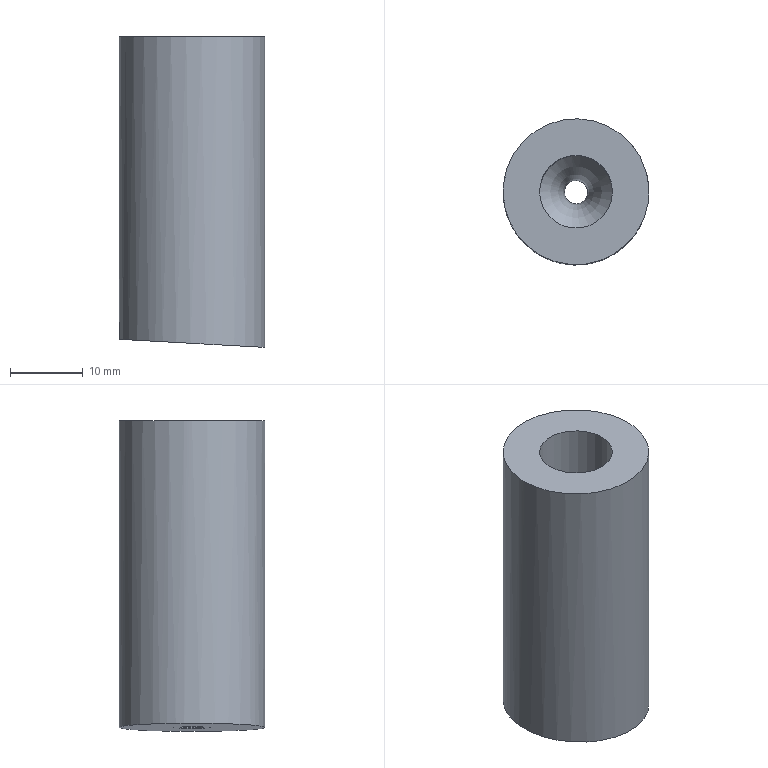Part | NX | features solid 2 | 1 solid | 7 faces | box 20 x 20 x 42.607 mm | volume 10571 mm3 | cylinder 3 | spline 2 | plane 1 | torus 1 | commonest cylinder face diameters 3.2 x1 10 x1 20 x1
STEP:
#1=CARTESIAN_POINT('',(262.245,42.7,-39.614));
#2=VERTEX_POINT('',#1);
#3=CARTESIAN_POINT('',(260.645,42.7,-39.614));
#4=DIRECTION('',(0.,0.,1.));
#5=DIRECTION('',(1.,0.,0.));
#6=AXIS2_PLACEMENT_3D('',#3,#4,#5);
#7=CIRCLE('',#6,1.6);
#8=EDGE_CURVE('',#2,#2,#7,.F.);
#9=ORIENTED_EDGE('',*,*,#8,.F.);
#10=EDGE_LOOP('',(#9));
#11=FACE_BOUND('',#10,.T.);
#12=CARTESIAN_POINT('',(260.645,44.3,-43.051));
#13=VERTEX_POINT('',#12);
#14=CARTESIAN_POINT('',(261.9,43.953,-43.121));
#15=CARTESIAN_POINT('',(260.645,44.473,-43.051));
#16=CARTESIAN_POINT('',(259.392,43.954,-42.982));
#17=CARTESIAN_POINT('',(258.872,42.701,-42.953));
#18=CARTESIAN_POINT('',(259.391,41.446,-42.982));
#19=CARTESIAN_POINT('',(260.645,40.927,-43.051));
#20=CARTESIAN_POINT('',(261.897,41.444,-43.121));
#21=CARTESIAN_POINT('',(262.419,42.698,-43.15));
#22=CARTESIAN_POINT('',(261.9,43.953,-43.121));
#23=CARTESIAN_POINT('',(260.645,44.473,-43.051));
#24=CARTESIAN_POINT('',(259.392,43.954,-42.982));
#25=B_SPLINE_CURVE_WITH_KNOTS('',3,(#14,#15,#16,#17,#18,#19,#20,#21,#22,#23,#24),.UNSPECIFIED.,.T.,.F.,(1,1,1,1,1,1,1,1,1,1,1,1,1,1,1),(-0.003754,-0.002503,-0.001251,0.,0.001251,0.002503,0.003754,0.005006,0.006257,0.007508,0.00876,0.01001,0.01126,0.01251,0.01377),.UNSPECIFIED.);
#26=EDGE_CURVE('',#13,#13,#25,.T.);
#27=ORIENTED_EDGE('',*,*,#26,.F.);
#28=EDGE_LOOP('',(#27));
#29=FACE_BOUND('',#28,.T.);
#30=CARTESIAN_POINT('',(260.645,42.7,-61.));
#31=DIRECTION('',(0.,0.,1.));
#32=DIRECTION('',(0.,1.,0.));
#33=AXIS2_PLACEMENT_3D('',#30,#31,#32);
#34=CYLINDRICAL_SURFACE('',#33,1.6);
#35=ADVANCED_FACE('',(#11,#29),#34,.F.);
#36=CARTESIAN_POINT('',(250.645,42.7,-1.));
#37=VERTEX_POINT('',#36);
#38=CARTESIAN_POINT('',(260.645,42.7,-1.));
#39=DIRECTION('',(0.,0.,-1.));
#40=DIRECTION('',(-1.,0.,0.));
#41=AXIS2_PLACEMENT_3D('',#38,#39,#40);
#42=CIRCLE('',#41,10.);
#43=EDGE_CURVE('',#37,#37,#42,.T.);
#44=ORIENTED_EDGE('',*,*,#43,.F.);
#45=EDGE_LOOP('',(#44));
#46=FACE_BOUND('',#45,.T.);
#47=CARTESIAN_POINT('',(255.645,42.7,-1.));
#48=VERTEX_POINT('',#47);
#49=CARTESIAN_POINT('',(260.645,42.7,-1.));
#50=DIRECTION('',(0.,0.,-1.));
#51=DIRECTION('',(-1.,0.,0.));
#52=AXIS2_PLACEMENT_3D('',#49,#50,#51);
#53=CIRCLE('',#52,5.);
#54=EDGE_CURVE('',#48,#48,#53,.F.);
#55=ORIENTED_EDGE('',*,*,#54,.F.);
#56=EDGE_LOOP('',(#55));
#57=FACE_BOUND('',#56,.T.);
#58=CARTESIAN_POINT('',(260.645,42.7,-1.));
#59=DIRECTION('',(0.,0.,-1.));
#60=DIRECTION('',(-1.,0.,0.));
#61=AXIS2_PLACEMENT_3D('',#58,#59,#60);
#62=PLANE('',#61);
#63=ADVANCED_FACE('',(#46,#57),#62,.F.);
#64=CARTESIAN_POINT('',(250.7,43.748,-42.499));
#65=VERTEX_POINT('',#64);
#66=CARTESIAN_POINT('',(253.686,51.326,-42.665));
#67=CARTESIAN_POINT('',(249.619,43.861,-42.439));
#68=CARTESIAN_POINT('',(252.038,35.721,-42.573));
#69=CARTESIAN_POINT('',(259.478,31.683,-42.986));
#70=CARTESIAN_POINT('',(267.608,34.077,-43.438));
#71=CARTESIAN_POINT('',(271.667,41.535,-43.664));
#72=CARTESIAN_POINT('',(269.262,49.666,-43.53));
#73=CARTESIAN_POINT('',(261.816,53.718,-43.116));
#74=CARTESIAN_POINT('',(253.686,51.326,-42.665));
#75=CARTESIAN_POINT('',(249.619,43.861,-42.439));
#76=CARTESIAN_POINT('',(252.038,35.721,-42.573));
#77=B_SPLINE_CURVE_WITH_KNOTS('',3,(#66,#67,#68,#69,#70,#71,#72,#73,#74,#75,#76),.UNSPECIFIED.,.T.,.F.,(1,1,1,1,1,1,1,1,1,1,1,1,1,1,1),(-0.02346,-0.01564,-0.007821,0.,0.007821,0.01564,0.02346,0.03129,0.03911,0.04693,0.05475,0.06257,0.07039,0.07821,0.08604),.UNSPECIFIED.);
#78=EDGE_CURVE('',#65,#65,#77,.T.);
#79=ORIENTED_EDGE('',*,*,#78,.T.);
#80=EDGE_LOOP('',(#79));
#81=FACE_BOUND('',#80,.T.);
#82=ORIENTED_EDGE('',*,*,#43,.T.);
#83=EDGE_LOOP('',(#82));
#84=FACE_BOUND('',#83,.T.);
#85=CARTESIAN_POINT('',(260.645,42.7,-51.));
#86=DIRECTION('',(0.,0.,1.));
#87=DIRECTION('',(1.,0.,0.));
#88=AXIS2_PLACEMENT_3D('',#85,#86,#87);
#89=CYLINDRICAL_SURFACE('',#88,10.);
#90=ADVANCED_FACE('',(#81,#84),#89,.T.);
#91=CARTESIAN_POINT('',(255.645,42.7,-31.705));
#92=VERTEX_POINT('',#91);
#93=CARTESIAN_POINT('',(260.645,42.7,-31.705));
#94=DIRECTION('',(0.,0.,-1.));
#95=DIRECTION('',(-1.,0.,0.));
#96=AXIS2_PLACEMENT_3D('',#93,#94,#95);
#97=CIRCLE('',#96,5.);
#98=EDGE_CURVE('',#92,#92,#97,.F.);
#99=ORIENTED_EDGE('',*,*,#98,.F.);
#100=EDGE_LOOP('',(#99));
#101=FACE_BOUND('',#100,.T.);
#102=ORIENTED_EDGE('',*,*,#54,.T.);
#103=EDGE_LOOP('',(#102));
#104=FACE_BOUND('',#103,.T.);
#105=CARTESIAN_POINT('',(260.645,42.7,29.));
#106=DIRECTION('',(0.,0.,-1.));
#107=DIRECTION('',(0.,-1.,0.));
#108=AXIS2_PLACEMENT_3D('',#105,#106,#107);
#109=CYLINDRICAL_SURFACE('',#108,5.);
#110=ADVANCED_FACE('',(#101,#104),#109,.F.);
#111=ORIENTED_EDGE('',*,*,#8,.T.);
#112=EDGE_LOOP('',(#111));
#113=FACE_BOUND('',#112,.T.);
#114=ORIENTED_EDGE('',*,*,#98,.T.);
#115=EDGE_LOOP('',(#114));
#116=FACE_BOUND('',#115,.T.);
#117=CARTESIAN_POINT('',(260.645,42.7,-39.614));
#118=DIRECTION('',(0.,0.,1.));
#119=DIRECTION('',(1.,0.,0.));
#120=AXIS2_PLACEMENT_3D('',#117,#118,#119);
#121=TOROIDAL_SURFACE('',#120,12.5,10.9);
#122=ADVANCED_FACE('',(#113,#116),#121,.T.);
#123=CARTESIAN_POINT('',(263.141,42.7,-43.19));
#124=VERTEX_POINT('',#123);
#125=CARTESIAN_POINT('',(258.148,42.7,-42.913));
#126=VERTEX_POINT('',#125);
#127=CARTESIAN_POINT('',(263.141,42.7,-43.19));
#128=CARTESIAN_POINT('',(263.14,43.391,-43.19));
#129=CARTESIAN_POINT('',(262.601,44.64,-43.16));
#130=CARTESIAN_POINT('',(260.644,45.48,-43.051));
#131=CARTESIAN_POINT('',(258.688,44.64,-42.943));
#132=CARTESIAN_POINT('',(258.148,43.39,-42.913));
#133=CARTESIAN_POINT('',(258.148,42.7,-42.913));
#134=B_SPLINE_CURVE_WITH_KNOTS('',3,(#127,#128,#129,#130,#131,#132,#133),.UNSPECIFIED.,.F.,.F.,(4,1,1,1,4),(0.,0.25,0.5,0.75,1.),.UNSPECIFIED.);
#135=EDGE_CURVE('',#124,#126,#134,.T.);
#136=ORIENTED_EDGE('',*,*,#135,.T.);
#137=CARTESIAN_POINT('',(258.148,42.7,-42.913));
#138=CARTESIAN_POINT('',(258.148,42.009,-42.913));
#139=CARTESIAN_POINT('',(258.688,40.76,-42.943));
#140=CARTESIAN_POINT('',(260.644,39.92,-43.051));
#141=CARTESIAN_POINT('',(262.6,40.759,-43.16));
#142=CARTESIAN_POINT('',(263.14,42.01,-43.19));
#143=CARTESIAN_POINT('',(263.141,42.7,-43.19));
#144=B_SPLINE_CURVE_WITH_KNOTS('',3,(#137,#138,#139,#140,#141,#142,#143),.UNSPECIFIED.,.F.,.F.,(4,1,1,1,4),(0.,0.25,0.5,0.75,1.),.UNSPECIFIED.);
#145=EDGE_CURVE('',#126,#124,#144,.T.);
#146=ORIENTED_EDGE('',*,*,#145,.T.);
#147=EDGE_LOOP('',(#136,#146));
#148=FACE_BOUND('',#147,.T.);
#149=ORIENTED_EDGE('',*,*,#78,.F.);
#150=EDGE_LOOP('',(#149));
#151=FACE_BOUND('',#150,.T.);
#152=CARTESIAN_POINT('',(250.462,52.882,-42.486));
#153=CARTESIAN_POINT('',(250.462,32.569,-42.486));
#154=CARTESIAN_POINT('',(250.834,52.882,-42.506));
#155=CARTESIAN_POINT('',(250.834,32.569,-42.506));
#156=CARTESIAN_POINT('',(270.827,52.882,-43.617));
#157=CARTESIAN_POINT('',(270.827,32.569,-43.617));
#158=B_SPLINE_SURFACE_WITH_KNOTS('',1,1,((#152,#153),(#154,#155),(#156,#157)),.PLANE_SURF.,.F.,.F.,.F.,(2,1,2),(2,2),(-0.01395,0.,0.7496),(0.6397,0.9362),.PIECEWISE_BEZIER_KNOTS.);
#159=ADVANCED_FACE('',(#148,#151),#158,.T.);
#160=ORIENTED_EDGE('',*,*,#145,.F.);
#161=ORIENTED_EDGE('',*,*,#135,.F.);
#162=EDGE_LOOP('',(#160,#161));
#163=FACE_BOUND('',#162,.T.);
#164=ORIENTED_EDGE('',*,*,#26,.T.);
#165=EDGE_LOOP('',(#164));
#166=FACE_BOUND('',#165,.T.);
#167=CARTESIAN_POINT('',(258.118,45.23,-42.911));
#168=CARTESIAN_POINT('',(258.118,40.17,-42.911));
#169=CARTESIAN_POINT('',(263.17,45.23,-43.192));
#170=CARTESIAN_POINT('',(263.17,40.17,-43.192));
#171=B_SPLINE_SURFACE_WITH_KNOTS('',1,1,((#167,#168),(#169,#170)),.PLANE_SURF.,.F.,.F.,.F.,(2,2),(2,2),(0.2731,0.4625),(0.7514,0.8253),.PIECEWISE_BEZIER_KNOTS.);
#172=ADVANCED_FACE('',(#163,#166),#171,.T.);
#173=CLOSED_SHELL('',(#35,#63,#90,#110,#122,#159,#172));
#174=MANIFOLD_SOLID_BREP('',#173);
#175=(LENGTH_UNIT()NAMED_UNIT(*)SI_UNIT(.MILLI.,.METRE.));
#176=UNCERTAINTY_MEASURE_WITH_UNIT(LENGTH_MEASURE(0.0508),#175,'','');
#177=(NAMED_UNIT(*)PLANE_ANGLE_UNIT()SI_UNIT($,.RADIAN.));
#178=(NAMED_UNIT(*)SI_UNIT($,.STERADIAN.)SOLID_ANGLE_UNIT());
#179=(GEOMETRIC_REPRESENTATION_CONTEXT(3)GLOBAL_UNCERTAINTY_ASSIGNED_CONTEXT((#176))GLOBAL_UNIT_ASSIGNED_CONTEXT((#175,#177,#178))REPRESENTATION_CONTEXT('',''));
#180=ADVANCED_BREP_SHAPE_REPRESENTATION('',(#174),#179);